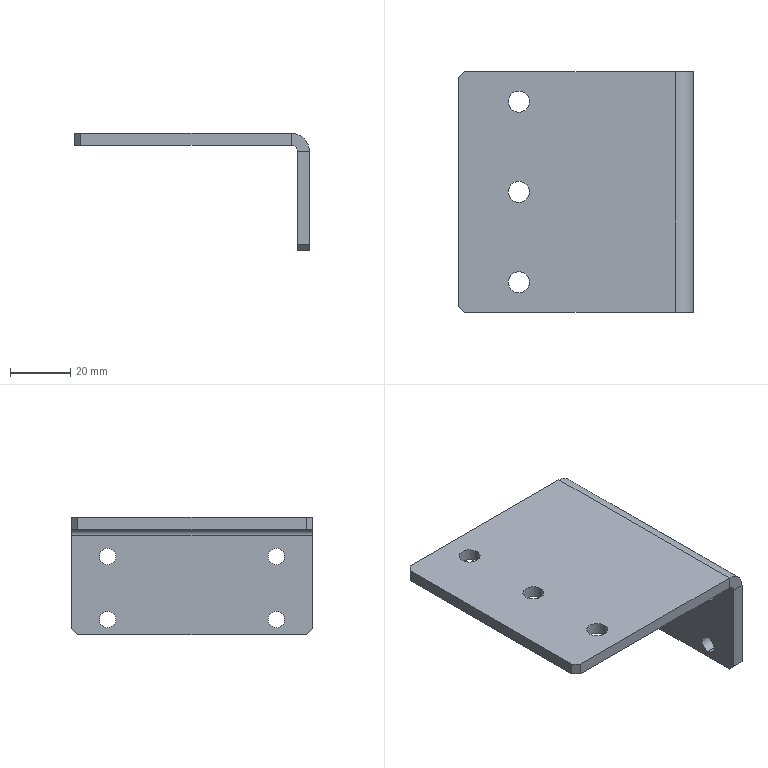Part | NX | features BREP 1 | 1 solid | 32 faces | box 78 x 80 x 39 mm | volume 34737 mm3 | plane 16 | cylinder 16 | commonest cylinder face diameters 5.5 x8 7 x6 4 x1 12 x1
STEP:
#1=CARTESIAN_POINT('',(74.,-38.,-35.));
#2=VERTEX_POINT('',#1);
#3=CARTESIAN_POINT('',(74.,-40.,-33.));
#4=VERTEX_POINT('',#3);
#5=CARTESIAN_POINT('',(74.,-16.5,-56.5));
#6=DIRECTION('',(0.,-0.7071,0.7071));
#7=VECTOR('',#6,1000.);
#8=LINE('',#5,#7);
#9=EDGE_CURVE('',#2,#4,#8,.T.);
#10=ORIENTED_EDGE('',*,*,#9,.F.);
#11=CARTESIAN_POINT('',(78.,-38.,-35.));
#12=VERTEX_POINT('',#11);
#13=CARTESIAN_POINT('',(74.,-38.,-35.));
#14=DIRECTION('',(-1.,0.,0.));
#15=VECTOR('',#14,1000.);
#16=LINE('',#13,#15);
#17=EDGE_CURVE('',#12,#2,#16,.T.);
#18=ORIENTED_EDGE('',*,*,#17,.F.);
#19=CARTESIAN_POINT('',(78.,-40.,-33.));
#20=VERTEX_POINT('',#19);
#21=CARTESIAN_POINT('',(78.,-40.,-33.));
#22=DIRECTION('',(0.,0.7071,-0.7071));
#23=VECTOR('',#22,1000.);
#24=LINE('',#21,#23);
#25=EDGE_CURVE('',#20,#12,#24,.T.);
#26=ORIENTED_EDGE('',*,*,#25,.F.);
#27=CARTESIAN_POINT('',(72.,-40.,-33.));
#28=DIRECTION('',(1.,0.,0.));
#29=VECTOR('',#28,1000.);
#30=LINE('',#27,#29);
#31=EDGE_CURVE('',#4,#20,#30,.T.);
#32=ORIENTED_EDGE('',*,*,#31,.F.);
#33=EDGE_LOOP('',(#10,#18,#26,#32));
#34=FACE_BOUND('',#33,.T.);
#35=CARTESIAN_POINT('',(72.,-40.,-33.));
#36=DIRECTION('',(0.,0.7071,0.7071));
#37=DIRECTION('',(1.,0.,0.));
#38=AXIS2_PLACEMENT_3D('',#35,#36,#37);
#39=PLANE('',#38);
#40=ADVANCED_FACE('',(#34),#39,.F.);
#41=CARTESIAN_POINT('',(74.,40.,-33.));
#42=VERTEX_POINT('',#41);
#43=CARTESIAN_POINT('',(74.,38.,-35.));
#44=VERTEX_POINT('',#43);
#45=CARTESIAN_POINT('',(74.,56.5,-16.5));
#46=DIRECTION('',(0.,-0.7071,-0.7071));
#47=VECTOR('',#46,1000.);
#48=LINE('',#45,#47);
#49=EDGE_CURVE('',#42,#44,#48,.T.);
#50=ORIENTED_EDGE('',*,*,#49,.F.);
#51=CARTESIAN_POINT('',(78.,40.,-33.));
#52=VERTEX_POINT('',#51);
#53=CARTESIAN_POINT('',(72.,40.,-33.));
#54=DIRECTION('',(-1.,0.,0.));
#55=VECTOR('',#54,1000.);
#56=LINE('',#53,#55);
#57=EDGE_CURVE('',#52,#42,#56,.T.);
#58=ORIENTED_EDGE('',*,*,#57,.F.);
#59=CARTESIAN_POINT('',(78.,38.,-35.));
#60=VERTEX_POINT('',#59);
#61=CARTESIAN_POINT('',(78.,38.,-35.));
#62=DIRECTION('',(0.,0.7071,0.7071));
#63=VECTOR('',#62,1000.);
#64=LINE('',#61,#63);
#65=EDGE_CURVE('',#60,#52,#64,.T.);
#66=ORIENTED_EDGE('',*,*,#65,.F.);
#67=CARTESIAN_POINT('',(74.,38.,-35.));
#68=DIRECTION('',(1.,0.,0.));
#69=VECTOR('',#68,1000.);
#70=LINE('',#67,#69);
#71=EDGE_CURVE('',#44,#60,#70,.T.);
#72=ORIENTED_EDGE('',*,*,#71,.F.);
#73=EDGE_LOOP('',(#50,#58,#66,#72));
#74=FACE_BOUND('',#73,.T.);
#75=CARTESIAN_POINT('',(74.,38.,-35.));
#76=DIRECTION('',(0.,-0.7071,0.7071));
#77=DIRECTION('',(1.,0.,0.));
#78=AXIS2_PLACEMENT_3D('',#75,#76,#77);
#79=PLANE('',#78);
#80=ADVANCED_FACE('',(#74),#79,.F.);
#81=CARTESIAN_POINT('',(0.,-38.,4.));
#82=VERTEX_POINT('',#81);
#83=CARTESIAN_POINT('',(2.,-40.,4.));
#84=VERTEX_POINT('',#83);
#85=CARTESIAN_POINT('',(2.,-40.,4.));
#86=DIRECTION('',(0.7071,-0.7071,0.));
#87=VECTOR('',#86,1000.);
#88=LINE('',#85,#87);
#89=EDGE_CURVE('',#82,#84,#88,.T.);
#90=ORIENTED_EDGE('',*,*,#89,.F.);
#91=CARTESIAN_POINT('',(0.,-38.,0.));
#92=VERTEX_POINT('',#91);
#93=CARTESIAN_POINT('',(0.,-38.,4.));
#94=DIRECTION('',(0.,0.,1.));
#95=VECTOR('',#94,1000.);
#96=LINE('',#93,#95);
#97=EDGE_CURVE('',#92,#82,#96,.T.);
#98=ORIENTED_EDGE('',*,*,#97,.F.);
#99=CARTESIAN_POINT('',(2.,-40.,0.));
#100=VERTEX_POINT('',#99);
#101=CARTESIAN_POINT('',(-39.,1.,0.));
#102=DIRECTION('',(-0.7071,0.7071,0.));
#103=VECTOR('',#102,1000.);
#104=LINE('',#101,#103);
#105=EDGE_CURVE('',#100,#92,#104,.T.);
#106=ORIENTED_EDGE('',*,*,#105,.F.);
#107=CARTESIAN_POINT('',(2.,-40.,-2.));
#108=DIRECTION('',(0.,0.,-1.));
#109=VECTOR('',#108,1000.);
#110=LINE('',#107,#109);
#111=EDGE_CURVE('',#84,#100,#110,.T.);
#112=ORIENTED_EDGE('',*,*,#111,.F.);
#113=EDGE_LOOP('',(#90,#98,#106,#112));
#114=FACE_BOUND('',#113,.T.);
#115=CARTESIAN_POINT('',(2.,-40.,-2.));
#116=DIRECTION('',(0.7071,0.7071,0.));
#117=DIRECTION('',(0.,0.,-1.));
#118=AXIS2_PLACEMENT_3D('',#115,#116,#117);
#119=PLANE('',#118);
#120=ADVANCED_FACE('',(#114),#119,.F.);
#121=CARTESIAN_POINT('',(2.,40.,4.));
#122=VERTEX_POINT('',#121);
#123=CARTESIAN_POINT('',(0.,38.,4.));
#124=VERTEX_POINT('',#123);
#125=CARTESIAN_POINT('',(0.,38.,4.));
#126=DIRECTION('',(-0.7071,-0.7071,0.));
#127=VECTOR('',#126,1000.);
#128=LINE('',#125,#127);
#129=EDGE_CURVE('',#122,#124,#128,.T.);
#130=ORIENTED_EDGE('',*,*,#129,.F.);
#131=CARTESIAN_POINT('',(2.,40.,0.));
#132=VERTEX_POINT('',#131);
#133=CARTESIAN_POINT('',(2.,40.,4.));
#134=DIRECTION('',(0.,0.,1.));
#135=VECTOR('',#134,1000.);
#136=LINE('',#133,#135);
#137=EDGE_CURVE('',#132,#122,#136,.T.);
#138=ORIENTED_EDGE('',*,*,#137,.F.);
#139=CARTESIAN_POINT('',(0.,38.,0.));
#140=VERTEX_POINT('',#139);
#141=CARTESIAN_POINT('',(1.,39.,0.));
#142=DIRECTION('',(0.7071,0.7071,0.));
#143=VECTOR('',#142,1000.);
#144=LINE('',#141,#143);
#145=EDGE_CURVE('',#140,#132,#144,.T.);
#146=ORIENTED_EDGE('',*,*,#145,.F.);
#147=CARTESIAN_POINT('',(0.,38.,0.));
#148=DIRECTION('',(0.,0.,-1.));
#149=VECTOR('',#148,1000.);
#150=LINE('',#147,#149);
#151=EDGE_CURVE('',#124,#140,#150,.T.);
#152=ORIENTED_EDGE('',*,*,#151,.F.);
#153=EDGE_LOOP('',(#130,#138,#146,#152));
#154=FACE_BOUND('',#153,.T.);
#155=CARTESIAN_POINT('',(0.,38.,4.));
#156=DIRECTION('',(-0.7071,0.7071,0.));
#157=DIRECTION('',(0.,0.,1.));
#158=AXIS2_PLACEMENT_3D('',#155,#156,#157);
#159=PLANE('',#158);
#160=ADVANCED_FACE('',(#154),#159,.T.);
#161=CARTESIAN_POINT('',(74.,28.,-6.25));
#162=VERTEX_POINT('',#161);
#163=CARTESIAN_POINT('',(78.,28.,-6.25));
#164=VERTEX_POINT('',#163);
#165=CARTESIAN_POINT('',(78.,28.,-6.25));
#166=DIRECTION('',(1.,0.,0.));
#167=VECTOR('',#166,1000.);
#168=LINE('',#165,#167);
#169=EDGE_CURVE('',#162,#164,#168,.T.);
#170=ORIENTED_EDGE('',*,*,#169,.F.);
#171=CARTESIAN_POINT('',(74.,28.,-11.75));
#172=VERTEX_POINT('',#171);
#173=CARTESIAN_POINT('',(74.,28.,-9.));
#174=DIRECTION('',(-1.,0.,0.));
#175=DIRECTION('',(0.,0.,1.));
#176=AXIS2_PLACEMENT_3D('',#173,#174,#175);
#177=CIRCLE('',#176,2.75);
#178=EDGE_CURVE('',#162,#172,#177,.T.);
#179=ORIENTED_EDGE('',*,*,#178,.T.);
#180=CARTESIAN_POINT('',(78.,28.,-11.75));
#181=VERTEX_POINT('',#180);
#182=CARTESIAN_POINT('',(78.,28.,-11.75));
#183=DIRECTION('',(1.,0.,0.));
#184=VECTOR('',#183,1000.);
#185=LINE('',#182,#184);
#186=EDGE_CURVE('',#172,#181,#185,.T.);
#187=ORIENTED_EDGE('',*,*,#186,.T.);
#188=CARTESIAN_POINT('',(78.,28.,-9.));
#189=DIRECTION('',(1.,0.,0.));
#190=DIRECTION('',(0.,0.,-1.));
#191=AXIS2_PLACEMENT_3D('',#188,#189,#190);
#192=CIRCLE('',#191,2.75);
#193=EDGE_CURVE('',#181,#164,#192,.T.);
#194=ORIENTED_EDGE('',*,*,#193,.T.);
#195=EDGE_LOOP('',(#170,#179,#187,#194));
#196=FACE_BOUND('',#195,.T.);
#197=CARTESIAN_POINT('',(78.,28.,-9.));
#198=DIRECTION('',(1.,0.,0.));
#199=DIRECTION('',(0.,0.,-1.));
#200=AXIS2_PLACEMENT_3D('',#197,#198,#199);
#201=CYLINDRICAL_SURFACE('',#200,2.75);
#202=ADVANCED_FACE('',(#196),#201,.F.);
#203=CARTESIAN_POINT('',(74.,28.,-27.25));
#204=VERTEX_POINT('',#203);
#205=CARTESIAN_POINT('',(78.,28.,-27.25));
#206=VERTEX_POINT('',#205);
#207=CARTESIAN_POINT('',(78.,28.,-27.25));
#208=DIRECTION('',(1.,0.,0.));
#209=VECTOR('',#208,1000.);
#210=LINE('',#207,#209);
#211=EDGE_CURVE('',#204,#206,#210,.T.);
#212=ORIENTED_EDGE('',*,*,#211,.F.);
#213=CARTESIAN_POINT('',(74.,28.,-32.75));
#214=VERTEX_POINT('',#213);
#215=CARTESIAN_POINT('',(74.,28.,-30.));
#216=DIRECTION('',(-1.,0.,0.));
#217=DIRECTION('',(0.,0.,1.));
#218=AXIS2_PLACEMENT_3D('',#215,#216,#217);
#219=CIRCLE('',#218,2.75);
#220=EDGE_CURVE('',#204,#214,#219,.T.);
#221=ORIENTED_EDGE('',*,*,#220,.T.);
#222=CARTESIAN_POINT('',(78.,28.,-32.75));
#223=VERTEX_POINT('',#222);
#224=CARTESIAN_POINT('',(78.,28.,-32.75));
#225=DIRECTION('',(1.,0.,0.));
#226=VECTOR('',#225,1000.);
#227=LINE('',#224,#226);
#228=EDGE_CURVE('',#214,#223,#227,.T.);
#229=ORIENTED_EDGE('',*,*,#228,.T.);
#230=CARTESIAN_POINT('',(78.,28.,-30.));
#231=DIRECTION('',(1.,0.,0.));
#232=DIRECTION('',(0.,0.,-1.));
#233=AXIS2_PLACEMENT_3D('',#230,#231,#232);
#234=CIRCLE('',#233,2.75);
#235=EDGE_CURVE('',#223,#206,#234,.T.);
#236=ORIENTED_EDGE('',*,*,#235,.T.);
#237=EDGE_LOOP('',(#212,#221,#229,#236));
#238=FACE_BOUND('',#237,.T.);
#239=CARTESIAN_POINT('',(78.,28.,-30.));
#240=DIRECTION('',(1.,0.,0.));
#241=DIRECTION('',(0.,0.,-1.));
#242=AXIS2_PLACEMENT_3D('',#239,#240,#241);
#243=CYLINDRICAL_SURFACE('',#242,2.75);
#244=ADVANCED_FACE('',(#238),#243,.F.);
#245=CARTESIAN_POINT('',(74.,-28.,-6.25));
#246=VERTEX_POINT('',#245);
#247=CARTESIAN_POINT('',(78.,-28.,-6.25));
#248=VERTEX_POINT('',#247);
#249=CARTESIAN_POINT('',(78.,-28.,-6.25));
#250=DIRECTION('',(1.,0.,0.));
#251=VECTOR('',#250,1000.);
#252=LINE('',#249,#251);
#253=EDGE_CURVE('',#246,#248,#252,.T.);
#254=ORIENTED_EDGE('',*,*,#253,.F.);
#255=CARTESIAN_POINT('',(74.,-28.,-11.75));
#256=VERTEX_POINT('',#255);
#257=CARTESIAN_POINT('',(74.,-28.,-9.));
#258=DIRECTION('',(-1.,0.,0.));
#259=DIRECTION('',(0.,0.,1.));
#260=AXIS2_PLACEMENT_3D('',#257,#258,#259);
#261=CIRCLE('',#260,2.75);
#262=EDGE_CURVE('',#246,#256,#261,.T.);
#263=ORIENTED_EDGE('',*,*,#262,.T.);
#264=CARTESIAN_POINT('',(78.,-28.,-11.75));
#265=VERTEX_POINT('',#264);
#266=CARTESIAN_POINT('',(78.,-28.,-11.75));
#267=DIRECTION('',(1.,0.,0.));
#268=VECTOR('',#267,1000.);
#269=LINE('',#266,#268);
#270=EDGE_CURVE('',#256,#265,#269,.T.);
#271=ORIENTED_EDGE('',*,*,#270,.T.);
#272=CARTESIAN_POINT('',(78.,-28.,-9.));
#273=DIRECTION('',(1.,0.,0.));
#274=DIRECTION('',(0.,0.,-1.));
#275=AXIS2_PLACEMENT_3D('',#272,#273,#274);
#276=CIRCLE('',#275,2.75);
#277=EDGE_CURVE('',#265,#248,#276,.T.);
#278=ORIENTED_EDGE('',*,*,#277,.T.);
#279=EDGE_LOOP('',(#254,#263,#271,#278));
#280=FACE_BOUND('',#279,.T.);
#281=CARTESIAN_POINT('',(78.,-28.,-9.));
#282=DIRECTION('',(1.,0.,0.));
#283=DIRECTION('',(0.,0.,-1.));
#284=AXIS2_PLACEMENT_3D('',#281,#282,#283);
#285=CYLINDRICAL_SURFACE('',#284,2.75);
#286=ADVANCED_FACE('',(#280),#285,.F.);
#287=CARTESIAN_POINT('',(74.,-28.,-27.25));
#288=VERTEX_POINT('',#287);
#289=CARTESIAN_POINT('',(78.,-28.,-27.25));
#290=VERTEX_POINT('',#289);
#291=CARTESIAN_POINT('',(78.,-28.,-27.25));
#292=DIRECTION('',(1.,0.,0.));
#293=VECTOR('',#292,1000.);
#294=LINE('',#291,#293);
#295=EDGE_CURVE('',#288,#290,#294,.T.);
#296=ORIENTED_EDGE('',*,*,#295,.F.);
#297=CARTESIAN_POINT('',(74.,-28.,-32.75));
#298=VERTEX_POINT('',#297);
#299=CARTESIAN_POINT('',(74.,-28.,-30.));
#300=DIRECTION('',(-1.,0.,0.));
#301=DIRECTION('',(0.,0.,1.));
#302=AXIS2_PLACEMENT_3D('',#299,#300,#301);
#303=CIRCLE('',#302,2.75);
#304=EDGE_CURVE('',#288,#298,#303,.T.);
#305=ORIENTED_EDGE('',*,*,#304,.T.);
#306=CARTESIAN_POINT('',(78.,-28.,-32.75));
#307=VERTEX_POINT('',#306);
#308=CARTESIAN_POINT('',(78.,-28.,-32.75));
#309=DIRECTION('',(1.,0.,0.));
#310=VECTOR('',#309,1000.);
#311=LINE('',#308,#310);
#312=EDGE_CURVE('',#298,#307,#311,.T.);
#313=ORIENTED_EDGE('',*,*,#312,.T.);
#314=CARTESIAN_POINT('',(78.,-28.,-30.));
#315=DIRECTION('',(1.,0.,0.));
#316=DIRECTION('',(0.,0.,-1.));
#317=AXIS2_PLACEMENT_3D('',#314,#315,#316);
#318=CIRCLE('',#317,2.75);
#319=EDGE_CURVE('',#307,#290,#318,.T.);
#320=ORIENTED_EDGE('',*,*,#319,.T.);
#321=EDGE_LOOP('',(#296,#305,#313,#320));
#322=FACE_BOUND('',#321,.T.);
#323=CARTESIAN_POINT('',(78.,-28.,-30.));
#324=DIRECTION('',(1.,0.,0.));
#325=DIRECTION('',(0.,0.,-1.));
#326=AXIS2_PLACEMENT_3D('',#323,#324,#325);
#327=CYLINDRICAL_SURFACE('',#326,2.75);
#328=ADVANCED_FACE('',(#322),#327,.F.);
#329=CARTESIAN_POINT('',(16.5,30.,4.));
#330=VERTEX_POINT('',#329);
#331=CARTESIAN_POINT('',(16.5,30.,0.));
#332=VERTEX_POINT('',#331);
#333=CARTESIAN_POINT('',(16.5,30.,4.));
#334=DIRECTION('',(0.,0.,1.));
#335=VECTOR('',#334,1000.);
#336=LINE('',#333,#335);
#337=EDGE_CURVE('',#330,#332,#336,.F.);
#338=ORIENTED_EDGE('',*,*,#337,.T.);
#339=CARTESIAN_POINT('',(23.5,30.,0.));
#340=VERTEX_POINT('',#339);
#341=CARTESIAN_POINT('',(20.,30.,0.));
#342=DIRECTION('',(0.,0.,-1.));
#343=DIRECTION('',(-1.,0.,0.));
#344=AXIS2_PLACEMENT_3D('',#341,#342,#343);
#345=CIRCLE('',#344,3.5);
#346=EDGE_CURVE('',#332,#340,#345,.T.);
#347=ORIENTED_EDGE('',*,*,#346,.T.);
#348=CARTESIAN_POINT('',(23.5,30.,4.));
#349=VERTEX_POINT('',#348);
#350=CARTESIAN_POINT('',(23.5,30.,4.));
#351=DIRECTION('',(0.,0.,1.));
#352=VECTOR('',#351,1000.);
#353=LINE('',#350,#352);
#354=EDGE_CURVE('',#349,#340,#353,.F.);
#355=ORIENTED_EDGE('',*,*,#354,.F.);
#356=CARTESIAN_POINT('',(20.,30.,4.));
#357=DIRECTION('',(0.,0.,1.));
#358=DIRECTION('',(1.,0.,0.));
#359=AXIS2_PLACEMENT_3D('',#356,#357,#358);
#360=CIRCLE('',#359,3.5);
#361=EDGE_CURVE('',#349,#330,#360,.T.);
#362=ORIENTED_EDGE('',*,*,#361,.T.);
#363=EDGE_LOOP('',(#338,#347,#355,#362));
#364=FACE_BOUND('',#363,.T.);
#365=CARTESIAN_POINT('',(20.,30.,4.));
#366=DIRECTION('',(0.,0.,1.));
#367=DIRECTION('',(1.,0.,0.));
#368=AXIS2_PLACEMENT_3D('',#365,#366,#367);
#369=CYLINDRICAL_SURFACE('',#368,3.5);
#370=ADVANCED_FACE('',(#364),#369,.F.);
#371=CARTESIAN_POINT('',(16.5,0.,4.));
#372=VERTEX_POINT('',#371);
#373=CARTESIAN_POINT('',(16.5,0.,0.));
#374=VERTEX_POINT('',#373);
#375=CARTESIAN_POINT('',(16.5,0.,4.));
#376=DIRECTION('',(0.,0.,1.));
#377=VECTOR('',#376,1000.);
#378=LINE('',#375,#377);
#379=EDGE_CURVE('',#372,#374,#378,.F.);
#380=ORIENTED_EDGE('',*,*,#379,.T.);
#381=CARTESIAN_POINT('',(23.5,0.,0.));
#382=VERTEX_POINT('',#381);
#383=CARTESIAN_POINT('',(20.,0.,0.));
#384=DIRECTION('',(0.,0.,-1.));
#385=DIRECTION('',(-1.,0.,0.));
#386=AXIS2_PLACEMENT_3D('',#383,#384,#385);
#387=CIRCLE('',#386,3.5);
#388=EDGE_CURVE('',#374,#382,#387,.T.);
#389=ORIENTED_EDGE('',*,*,#388,.T.);
#390=CARTESIAN_POINT('',(23.5,0.,4.));
#391=VERTEX_POINT('',#390);
#392=CARTESIAN_POINT('',(23.5,0.,4.));
#393=DIRECTION('',(0.,0.,1.));
#394=VECTOR('',#393,1000.);
#395=LINE('',#392,#394);
#396=EDGE_CURVE('',#391,#382,#395,.F.);
#397=ORIENTED_EDGE('',*,*,#396,.F.);
#398=CARTESIAN_POINT('',(20.,0.,4.));
#399=DIRECTION('',(0.,0.,1.));
#400=DIRECTION('',(1.,0.,0.));
#401=AXIS2_PLACEMENT_3D('',#398,#399,#400);
#402=CIRCLE('',#401,3.5);
#403=EDGE_CURVE('',#391,#372,#402,.T.);
#404=ORIENTED_EDGE('',*,*,#403,.T.);
#405=EDGE_LOOP('',(#380,#389,#397,#404));
#406=FACE_BOUND('',#405,.T.);
#407=CARTESIAN_POINT('',(20.,0.,4.));
#408=DIRECTION('',(0.,0.,1.));
#409=DIRECTION('',(1.,0.,0.));
#410=AXIS2_PLACEMENT_3D('',#407,#408,#409);
#411=CYLINDRICAL_SURFACE('',#410,3.5);
#412=ADVANCED_FACE('',(#406),#411,.F.);
#413=CARTESIAN_POINT('',(16.5,-30.,4.));
#414=VERTEX_POINT('',#413);
#415=CARTESIAN_POINT('',(16.5,-30.,0.));
#416=VERTEX_POINT('',#415);
#417=CARTESIAN_POINT('',(16.5,-30.,4.));
#418=DIRECTION('',(0.,0.,1.));
#419=VECTOR('',#418,1000.);
#420=LINE('',#417,#419);
#421=EDGE_CURVE('',#414,#416,#420,.F.);
#422=ORIENTED_EDGE('',*,*,#421,.T.);
#423=CARTESIAN_POINT('',(23.5,-30.,0.));
#424=VERTEX_POINT('',#423);
#425=CARTESIAN_POINT('',(20.,-30.,0.));
#426=DIRECTION('',(0.,0.,-1.));
#427=DIRECTION('',(-1.,0.,0.));
#428=AXIS2_PLACEMENT_3D('',#425,#426,#427);
#429=CIRCLE('',#428,3.5);
#430=EDGE_CURVE('',#416,#424,#429,.T.);
#431=ORIENTED_EDGE('',*,*,#430,.T.);
#432=CARTESIAN_POINT('',(23.5,-30.,4.));
#433=VERTEX_POINT('',#432);
#434=CARTESIAN_POINT('',(23.5,-30.,4.));
#435=DIRECTION('',(0.,0.,1.));
#436=VECTOR('',#435,1000.);
#437=LINE('',#434,#436);
#438=EDGE_CURVE('',#433,#424,#437,.F.);
#439=ORIENTED_EDGE('',*,*,#438,.F.);
#440=CARTESIAN_POINT('',(20.,-30.,4.));
#441=DIRECTION('',(0.,0.,1.));
#442=DIRECTION('',(1.,0.,0.));
#443=AXIS2_PLACEMENT_3D('',#440,#441,#442);
#444=CIRCLE('',#443,3.5);
#445=EDGE_CURVE('',#433,#414,#444,.T.);
#446=ORIENTED_EDGE('',*,*,#445,.T.);
#447=EDGE_LOOP('',(#422,#431,#439,#446));
#448=FACE_BOUND('',#447,.T.);
#449=CARTESIAN_POINT('',(20.,-30.,4.));
#450=DIRECTION('',(0.,0.,1.));
#451=DIRECTION('',(1.,0.,0.));
#452=AXIS2_PLACEMENT_3D('',#449,#450,#451);
#453=CYLINDRICAL_SURFACE('',#452,3.5);
#454=ADVANCED_FACE('',(#448),#453,.F.);
#455=CARTESIAN_POINT('',(74.,-40.,-2.));
#456=VERTEX_POINT('',#455);
#457=CARTESIAN_POINT('',(74.,-40.,0.));
#458=DIRECTION('',(0.,0.,-1.));
#459=VECTOR('',#458,1000.);
#460=LINE('',#457,#459);
#461=EDGE_CURVE('',#456,#4,#460,.T.);
#462=ORIENTED_EDGE('',*,*,#461,.T.);
#463=ORIENTED_EDGE('',*,*,#31,.T.);
#464=CARTESIAN_POINT('',(78.,-40.,-2.));
#465=VERTEX_POINT('',#464);
#466=CARTESIAN_POINT('',(78.,-40.,0.));
#467=DIRECTION('',(0.,0.,-1.));
#468=VECTOR('',#467,1000.);
#469=LINE('',#466,#468);
#470=EDGE_CURVE('',#465,#20,#469,.T.);
#471=ORIENTED_EDGE('',*,*,#470,.F.);
#472=CARTESIAN_POINT('',(78.,-40.,-2.));
#473=DIRECTION('',(-1.,0.,0.));
#474=VECTOR('',#473,1000.);
#475=LINE('',#472,#474);
#476=EDGE_CURVE('',#465,#456,#475,.T.);
#477=ORIENTED_EDGE('',*,*,#476,.T.);
#478=EDGE_LOOP('',(#462,#463,#471,#477));
#479=FACE_BOUND('',#478,.T.);
#480=CARTESIAN_POINT('',(72.,-40.,-2.));
#481=DIRECTION('',(0.,-1.,0.));
#482=DIRECTION('',(-1.,0.,0.));
#483=AXIS2_PLACEMENT_3D('',#480,#481,#482);
#484=PLANE('',#483);
#485=ADVANCED_FACE('',(#479),#484,.T.);
#486=CARTESIAN_POINT('',(72.,40.,0.));
#487=VERTEX_POINT('',#486);
#488=CARTESIAN_POINT('',(0.,40.,0.));
#489=DIRECTION('',(1.,0.,0.));
#490=VECTOR('',#489,1000.);
#491=LINE('',#488,#490);
#492=EDGE_CURVE('',#132,#487,#491,.T.);
#493=ORIENTED_EDGE('',*,*,#492,.F.);
#494=ORIENTED_EDGE('',*,*,#137,.T.);
#495=CARTESIAN_POINT('',(72.,40.,4.));
#496=VERTEX_POINT('',#495);
#497=CARTESIAN_POINT('',(0.,40.,4.));
#498=DIRECTION('',(1.,0.,0.));
#499=VECTOR('',#498,1000.);
#500=LINE('',#497,#499);
#501=EDGE_CURVE('',#122,#496,#500,.T.);
#502=ORIENTED_EDGE('',*,*,#501,.T.);
#503=CARTESIAN_POINT('',(72.,40.,4.));
#504=DIRECTION('',(0.,0.,-1.));
#505=VECTOR('',#504,1000.);
#506=LINE('',#503,#505);
#507=EDGE_CURVE('',#496,#487,#506,.T.);
#508=ORIENTED_EDGE('',*,*,#507,.T.);
#509=EDGE_LOOP('',(#493,#494,#502,#508));
#510=FACE_BOUND('',#509,.T.);
#511=CARTESIAN_POINT('',(72.,40.,-2.));
#512=DIRECTION('',(0.,-1.,0.));
#513=DIRECTION('',(-1.,0.,0.));
#514=AXIS2_PLACEMENT_3D('',#511,#512,#513);
#515=PLANE('',#514);
#516=ADVANCED_FACE('',(#510),#515,.F.);
#517=CARTESIAN_POINT('',(72.,-40.,4.));
#518=VERTEX_POINT('',#517);
#519=CARTESIAN_POINT('',(72.,-40.,-2.));
#520=DIRECTION('',(0.,1.,0.));
#521=DIRECTION('',(1.,0.,0.));
#522=AXIS2_PLACEMENT_3D('',#519,#520,#521);
#523=CIRCLE('',#522,6.);
#524=EDGE_CURVE('',#518,#465,#523,.T.);
#525=ORIENTED_EDGE('',*,*,#524,.T.);
#526=CARTESIAN_POINT('',(78.,40.,-2.));
#527=VERTEX_POINT('',#526);
#528=CARTESIAN_POINT('',(78.,40.,-2.));
#529=DIRECTION('',(0.,-1.,0.));
#530=VECTOR('',#529,1000.);
#531=LINE('',#528,#530);
#532=EDGE_CURVE('',#527,#465,#531,.T.);
#533=ORIENTED_EDGE('',*,*,#532,.F.);
#534=CARTESIAN_POINT('',(72.,40.,-2.));
#535=DIRECTION('',(0.,1.,0.));
#536=DIRECTION('',(1.,0.,0.));
#537=AXIS2_PLACEMENT_3D('',#534,#535,#536);
#538=CIRCLE('',#537,6.);
#539=EDGE_CURVE('',#496,#527,#538,.T.);
#540=ORIENTED_EDGE('',*,*,#539,.F.);
#541=CARTESIAN_POINT('',(72.,40.,4.));
#542=DIRECTION('',(0.,-1.,0.));
#543=VECTOR('',#542,1000.);
#544=LINE('',#541,#543);
#545=EDGE_CURVE('',#496,#518,#544,.T.);
#546=ORIENTED_EDGE('',*,*,#545,.T.);
#547=EDGE_LOOP('',(#525,#533,#540,#546));
#548=FACE_BOUND('',#547,.T.);
#549=CARTESIAN_POINT('',(72.,40.,-2.));
#550=DIRECTION('',(0.,-1.,0.));
#551=DIRECTION('',(0.,0.,-1.));
#552=AXIS2_PLACEMENT_3D('',#549,#550,#551);
#553=CYLINDRICAL_SURFACE('',#552,6.);
#554=ADVANCED_FACE('',(#548),#553,.T.);
#555=ORIENTED_EDGE('',*,*,#501,.F.);
#556=ORIENTED_EDGE('',*,*,#129,.T.);
#557=CARTESIAN_POINT('',(0.,40.,4.));
#558=DIRECTION('',(0.,-1.,0.));
#559=VECTOR('',#558,1000.);
#560=LINE('',#557,#559);
#561=EDGE_CURVE('',#124,#82,#560,.T.);
#562=ORIENTED_EDGE('',*,*,#561,.T.);
#563=ORIENTED_EDGE('',*,*,#89,.T.);
#564=CARTESIAN_POINT('',(0.,-40.,4.));
#565=DIRECTION('',(1.,0.,0.));
#566=VECTOR('',#565,1000.);
#567=LINE('',#564,#566);
#568=EDGE_CURVE('',#84,#518,#567,.T.);
#569=ORIENTED_EDGE('',*,*,#568,.T.);
#570=ORIENTED_EDGE('',*,*,#545,.F.);
#571=EDGE_LOOP('',(#555,#556,#562,#563,#569,#570));
#572=FACE_BOUND('',#571,.T.);
#573=ORIENTED_EDGE('',*,*,#445,.F.);
#574=CARTESIAN_POINT('',(20.,-30.,4.));
#575=DIRECTION('',(0.,0.,1.));
#576=DIRECTION('',(1.,0.,0.));
#577=AXIS2_PLACEMENT_3D('',#574,#575,#576);
#578=CIRCLE('',#577,3.5);
#579=EDGE_CURVE('',#414,#433,#578,.T.);
#580=ORIENTED_EDGE('',*,*,#579,.F.);
#581=EDGE_LOOP('',(#573,#580));
#582=FACE_BOUND('',#581,.T.);
#583=ORIENTED_EDGE('',*,*,#403,.F.);
#584=CARTESIAN_POINT('',(20.,0.,4.));
#585=DIRECTION('',(0.,0.,1.));
#586=DIRECTION('',(1.,0.,0.));
#587=AXIS2_PLACEMENT_3D('',#584,#585,#586);
#588=CIRCLE('',#587,3.5);
#589=EDGE_CURVE('',#372,#391,#588,.T.);
#590=ORIENTED_EDGE('',*,*,#589,.F.);
#591=EDGE_LOOP('',(#583,#590));
#592=FACE_BOUND('',#591,.T.);
#593=ORIENTED_EDGE('',*,*,#361,.F.);
#594=CARTESIAN_POINT('',(20.,30.,4.));
#595=DIRECTION('',(0.,0.,1.));
#596=DIRECTION('',(1.,0.,0.));
#597=AXIS2_PLACEMENT_3D('',#594,#595,#596);
#598=CIRCLE('',#597,3.5);
#599=EDGE_CURVE('',#330,#349,#598,.T.);
#600=ORIENTED_EDGE('',*,*,#599,.F.);
#601=EDGE_LOOP('',(#593,#600));
#602=FACE_BOUND('',#601,.T.);
#603=CARTESIAN_POINT('',(0.,40.,4.));
#604=DIRECTION('',(0.,0.,-1.));
#605=DIRECTION('',(-1.,0.,0.));
#606=AXIS2_PLACEMENT_3D('',#603,#604,#605);
#607=PLANE('',#606);
#608=ADVANCED_FACE('',(#572,#582,#592,#602),#607,.F.);
#609=ORIENTED_EDGE('',*,*,#561,.F.);
#610=ORIENTED_EDGE('',*,*,#151,.T.);
#611=CARTESIAN_POINT('',(0.,40.,0.));
#612=DIRECTION('',(0.,-1.,0.));
#613=VECTOR('',#612,1000.);
#614=LINE('',#611,#613);
#615=EDGE_CURVE('',#140,#92,#614,.T.);
#616=ORIENTED_EDGE('',*,*,#615,.T.);
#617=ORIENTED_EDGE('',*,*,#97,.T.);
#618=EDGE_LOOP('',(#609,#610,#616,#617));
#619=FACE_BOUND('',#618,.T.);
#620=CARTESIAN_POINT('',(0.,40.,4.));
#621=DIRECTION('',(-1.,0.,0.));
#622=DIRECTION('',(0.,0.,1.));
#623=AXIS2_PLACEMENT_3D('',#620,#621,#622);
#624=PLANE('',#623);
#625=ADVANCED_FACE('',(#619),#624,.T.);
#626=ORIENTED_EDGE('',*,*,#615,.F.);
#627=ORIENTED_EDGE('',*,*,#145,.T.);
#628=ORIENTED_EDGE('',*,*,#492,.T.);
#629=CARTESIAN_POINT('',(72.,-40.,0.));
#630=VERTEX_POINT('',#629);
#631=CARTESIAN_POINT('',(72.,40.,0.));
#632=DIRECTION('',(0.,-1.,0.));
#633=VECTOR('',#632,1000.);
#634=LINE('',#631,#633);
#635=EDGE_CURVE('',#487,#630,#634,.T.);
#636=ORIENTED_EDGE('',*,*,#635,.T.);
#637=CARTESIAN_POINT('',(0.,-40.,0.));
#638=DIRECTION('',(1.,0.,0.));
#639=VECTOR('',#638,1000.);
#640=LINE('',#637,#639);
#641=EDGE_CURVE('',#100,#630,#640,.T.);
#642=ORIENTED_EDGE('',*,*,#641,.F.);
#643=ORIENTED_EDGE('',*,*,#105,.T.);
#644=EDGE_LOOP('',(#626,#627,#628,#636,#642,#643));
#645=FACE_BOUND('',#644,.T.);
#646=CARTESIAN_POINT('',(20.,-30.,0.));
#647=DIRECTION('',(0.,0.,-1.));
#648=DIRECTION('',(-1.,0.,0.));
#649=AXIS2_PLACEMENT_3D('',#646,#647,#648);
#650=CIRCLE('',#649,3.5);
#651=EDGE_CURVE('',#424,#416,#650,.T.);
#652=ORIENTED_EDGE('',*,*,#651,.F.);
#653=ORIENTED_EDGE('',*,*,#430,.F.);
#654=EDGE_LOOP('',(#652,#653));
#655=FACE_BOUND('',#654,.T.);
#656=CARTESIAN_POINT('',(20.,0.,0.));
#657=DIRECTION('',(0.,0.,-1.));
#658=DIRECTION('',(-1.,0.,0.));
#659=AXIS2_PLACEMENT_3D('',#656,#657,#658);
#660=CIRCLE('',#659,3.5);
#661=EDGE_CURVE('',#382,#374,#660,.T.);
#662=ORIENTED_EDGE('',*,*,#661,.F.);
#663=ORIENTED_EDGE('',*,*,#388,.F.);
#664=EDGE_LOOP('',(#662,#663));
#665=FACE_BOUND('',#664,.T.);
#666=CARTESIAN_POINT('',(20.,30.,0.));
#667=DIRECTION('',(0.,0.,-1.));
#668=DIRECTION('',(-1.,0.,0.));
#669=AXIS2_PLACEMENT_3D('',#666,#667,#668);
#670=CIRCLE('',#669,3.5);
#671=EDGE_CURVE('',#340,#332,#670,.T.);
#672=ORIENTED_EDGE('',*,*,#671,.F.);
#673=ORIENTED_EDGE('',*,*,#346,.F.);
#674=EDGE_LOOP('',(#672,#673));
#675=FACE_BOUND('',#674,.T.);
#676=CARTESIAN_POINT('',(0.,40.,0.));
#677=DIRECTION('',(0.,0.,-1.));
#678=DIRECTION('',(-1.,0.,0.));
#679=AXIS2_PLACEMENT_3D('',#676,#677,#678);
#680=PLANE('',#679);
#681=ADVANCED_FACE('',(#645,#655,#665,#675),#680,.T.);
#682=CARTESIAN_POINT('',(72.,-40.,-2.));
#683=DIRECTION('',(0.,1.,0.));
#684=DIRECTION('',(0.,0.,-1.));
#685=AXIS2_PLACEMENT_3D('',#682,#683,#684);
#686=CIRCLE('',#685,2.);
#687=EDGE_CURVE('',#630,#456,#686,.T.);
#688=ORIENTED_EDGE('',*,*,#687,.F.);
#689=ORIENTED_EDGE('',*,*,#635,.F.);
#690=CARTESIAN_POINT('',(74.,40.,-2.));
#691=VERTEX_POINT('',#690);
#692=CARTESIAN_POINT('',(72.,40.,-2.));
#693=DIRECTION('',(0.,1.,0.));
#694=DIRECTION('',(0.,0.,-1.));
#695=AXIS2_PLACEMENT_3D('',#692,#693,#694);
#696=CIRCLE('',#695,2.);
#697=EDGE_CURVE('',#487,#691,#696,.T.);
#698=ORIENTED_EDGE('',*,*,#697,.T.);
#699=CARTESIAN_POINT('',(74.,40.,-2.));
#700=DIRECTION('',(0.,-1.,0.));
#701=VECTOR('',#700,1000.);
#702=LINE('',#699,#701);
#703=EDGE_CURVE('',#691,#456,#702,.T.);
#704=ORIENTED_EDGE('',*,*,#703,.T.);
#705=EDGE_LOOP('',(#688,#689,#698,#704));
#706=FACE_BOUND('',#705,.T.);
#707=CARTESIAN_POINT('',(72.,40.,-2.));
#708=DIRECTION('',(0.,-1.,0.));
#709=DIRECTION('',(0.,0.,-1.));
#710=AXIS2_PLACEMENT_3D('',#707,#708,#709);
#711=CYLINDRICAL_SURFACE('',#710,2.);
#712=ADVANCED_FACE('',(#706),#711,.F.);
#713=CARTESIAN_POINT('',(74.,40.,0.));
#714=DIRECTION('',(0.,0.,-1.));
#715=VECTOR('',#714,1000.);
#716=LINE('',#713,#715);
#717=EDGE_CURVE('',#691,#42,#716,.T.);
#718=ORIENTED_EDGE('',*,*,#717,.T.);
#719=ORIENTED_EDGE('',*,*,#49,.T.);
#720=CARTESIAN_POINT('',(74.,40.,-35.));
#721=DIRECTION('',(0.,-1.,0.));
#722=VECTOR('',#721,1000.);
#723=LINE('',#720,#722);
#724=EDGE_CURVE('',#44,#2,#723,.T.);
#725=ORIENTED_EDGE('',*,*,#724,.T.);
#726=ORIENTED_EDGE('',*,*,#9,.T.);
#727=ORIENTED_EDGE('',*,*,#461,.F.);
#728=ORIENTED_EDGE('',*,*,#703,.F.);
#729=EDGE_LOOP('',(#718,#719,#725,#726,#727,#728));
#730=FACE_BOUND('',#729,.T.);
#731=CARTESIAN_POINT('',(74.,-28.,-30.));
#732=DIRECTION('',(-1.,0.,0.));
#733=DIRECTION('',(0.,0.,1.));
#734=AXIS2_PLACEMENT_3D('',#731,#732,#733);
#735=CIRCLE('',#734,2.75);
#736=EDGE_CURVE('',#298,#288,#735,.T.);
#737=ORIENTED_EDGE('',*,*,#736,.F.);
#738=ORIENTED_EDGE('',*,*,#304,.F.);
#739=EDGE_LOOP('',(#737,#738));
#740=FACE_BOUND('',#739,.T.);
#741=CARTESIAN_POINT('',(74.,-28.,-9.));
#742=DIRECTION('',(-1.,0.,0.));
#743=DIRECTION('',(0.,0.,1.));
#744=AXIS2_PLACEMENT_3D('',#741,#742,#743);
#745=CIRCLE('',#744,2.75);
#746=EDGE_CURVE('',#256,#246,#745,.T.);
#747=ORIENTED_EDGE('',*,*,#746,.F.);
#748=ORIENTED_EDGE('',*,*,#262,.F.);
#749=EDGE_LOOP('',(#747,#748));
#750=FACE_BOUND('',#749,.T.);
#751=CARTESIAN_POINT('',(74.,28.,-30.));
#752=DIRECTION('',(-1.,0.,0.));
#753=DIRECTION('',(0.,0.,1.));
#754=AXIS2_PLACEMENT_3D('',#751,#752,#753);
#755=CIRCLE('',#754,2.75);
#756=EDGE_CURVE('',#214,#204,#755,.T.);
#757=ORIENTED_EDGE('',*,*,#756,.F.);
#758=ORIENTED_EDGE('',*,*,#220,.F.);
#759=EDGE_LOOP('',(#757,#758));
#760=FACE_BOUND('',#759,.T.);
#761=CARTESIAN_POINT('',(74.,28.,-9.));
#762=DIRECTION('',(-1.,0.,0.));
#763=DIRECTION('',(0.,0.,1.));
#764=AXIS2_PLACEMENT_3D('',#761,#762,#763);
#765=CIRCLE('',#764,2.75);
#766=EDGE_CURVE('',#172,#162,#765,.T.);
#767=ORIENTED_EDGE('',*,*,#766,.F.);
#768=ORIENTED_EDGE('',*,*,#178,.F.);
#769=EDGE_LOOP('',(#767,#768));
#770=FACE_BOUND('',#769,.T.);
#771=CARTESIAN_POINT('',(74.,40.,0.));
#772=DIRECTION('',(-1.,0.,0.));
#773=DIRECTION('',(0.,0.,1.));
#774=AXIS2_PLACEMENT_3D('',#771,#772,#773);
#775=PLANE('',#774);
#776=ADVANCED_FACE('',(#730,#740,#750,#760,#770),#775,.T.);
#777=ORIENTED_EDGE('',*,*,#724,.F.);
#778=ORIENTED_EDGE('',*,*,#71,.T.);
#779=CARTESIAN_POINT('',(78.,40.,-35.));
#780=DIRECTION('',(0.,-1.,0.));
#781=VECTOR('',#780,1000.);
#782=LINE('',#779,#781);
#783=EDGE_CURVE('',#60,#12,#782,.T.);
#784=ORIENTED_EDGE('',*,*,#783,.T.);
#785=ORIENTED_EDGE('',*,*,#17,.T.);
#786=EDGE_LOOP('',(#777,#778,#784,#785));
#787=FACE_BOUND('',#786,.T.);
#788=CARTESIAN_POINT('',(74.,40.,-35.));
#789=DIRECTION('',(0.,0.,-1.));
#790=DIRECTION('',(-1.,0.,0.));
#791=AXIS2_PLACEMENT_3D('',#788,#789,#790);
#792=PLANE('',#791);
#793=ADVANCED_FACE('',(#787),#792,.T.);
#794=ORIENTED_EDGE('',*,*,#783,.F.);
#795=ORIENTED_EDGE('',*,*,#65,.T.);
#796=CARTESIAN_POINT('',(78.,40.,0.));
#797=DIRECTION('',(0.,0.,-1.));
#798=VECTOR('',#797,1000.);
#799=LINE('',#796,#798);
#800=EDGE_CURVE('',#527,#52,#799,.T.);
#801=ORIENTED_EDGE('',*,*,#800,.F.);
#802=ORIENTED_EDGE('',*,*,#532,.T.);
#803=ORIENTED_EDGE('',*,*,#470,.T.);
#804=ORIENTED_EDGE('',*,*,#25,.T.);
#805=EDGE_LOOP('',(#794,#795,#801,#802,#803,#804));
#806=FACE_BOUND('',#805,.T.);
#807=ORIENTED_EDGE('',*,*,#319,.F.);
#808=CARTESIAN_POINT('',(78.,-28.,-30.));
#809=DIRECTION('',(1.,0.,0.));
#810=DIRECTION('',(0.,0.,-1.));
#811=AXIS2_PLACEMENT_3D('',#808,#809,#810);
#812=CIRCLE('',#811,2.75);
#813=EDGE_CURVE('',#290,#307,#812,.T.);
#814=ORIENTED_EDGE('',*,*,#813,.F.);
#815=EDGE_LOOP('',(#807,#814));
#816=FACE_BOUND('',#815,.T.);
#817=ORIENTED_EDGE('',*,*,#277,.F.);
#818=CARTESIAN_POINT('',(78.,-28.,-9.));
#819=DIRECTION('',(1.,0.,0.));
#820=DIRECTION('',(0.,0.,-1.));
#821=AXIS2_PLACEMENT_3D('',#818,#819,#820);
#822=CIRCLE('',#821,2.75);
#823=EDGE_CURVE('',#248,#265,#822,.T.);
#824=ORIENTED_EDGE('',*,*,#823,.F.);
#825=EDGE_LOOP('',(#817,#824));
#826=FACE_BOUND('',#825,.T.);
#827=ORIENTED_EDGE('',*,*,#235,.F.);
#828=CARTESIAN_POINT('',(78.,28.,-30.));
#829=DIRECTION('',(1.,0.,0.));
#830=DIRECTION('',(0.,0.,-1.));
#831=AXIS2_PLACEMENT_3D('',#828,#829,#830);
#832=CIRCLE('',#831,2.75);
#833=EDGE_CURVE('',#206,#223,#832,.T.);
#834=ORIENTED_EDGE('',*,*,#833,.F.);
#835=EDGE_LOOP('',(#827,#834));
#836=FACE_BOUND('',#835,.T.);
#837=ORIENTED_EDGE('',*,*,#193,.F.);
#838=CARTESIAN_POINT('',(78.,28.,-9.));
#839=DIRECTION('',(1.,0.,0.));
#840=DIRECTION('',(0.,0.,-1.));
#841=AXIS2_PLACEMENT_3D('',#838,#839,#840);
#842=CIRCLE('',#841,2.75);
#843=EDGE_CURVE('',#164,#181,#842,.T.);
#844=ORIENTED_EDGE('',*,*,#843,.F.);
#845=EDGE_LOOP('',(#837,#844));
#846=FACE_BOUND('',#845,.T.);
#847=CARTESIAN_POINT('',(78.,40.,0.));
#848=DIRECTION('',(-1.,0.,0.));
#849=DIRECTION('',(0.,0.,1.));
#850=AXIS2_PLACEMENT_3D('',#847,#848,#849);
#851=PLANE('',#850);
#852=ADVANCED_FACE('',(#806,#816,#826,#836,#846),#851,.F.);
#853=ORIENTED_EDGE('',*,*,#568,.F.);
#854=ORIENTED_EDGE('',*,*,#111,.T.);
#855=ORIENTED_EDGE('',*,*,#641,.T.);
#856=CARTESIAN_POINT('',(72.,-40.,0.));
#857=DIRECTION('',(0.,0.,1.));
#858=VECTOR('',#857,1000.);
#859=LINE('',#856,#858);
#860=EDGE_CURVE('',#630,#518,#859,.T.);
#861=ORIENTED_EDGE('',*,*,#860,.T.);
#862=EDGE_LOOP('',(#853,#854,#855,#861));
#863=FACE_BOUND('',#862,.T.);
#864=CARTESIAN_POINT('',(78.,-40.,-2.));
#865=DIRECTION('',(0.,-1.,0.));
#866=DIRECTION('',(0.,0.,-1.));
#867=AXIS2_PLACEMENT_3D('',#864,#865,#866);
#868=PLANE('',#867);
#869=ADVANCED_FACE('',(#863),#868,.T.);
#870=ORIENTED_EDGE('',*,*,#860,.F.);
#871=ORIENTED_EDGE('',*,*,#687,.T.);
#872=ORIENTED_EDGE('',*,*,#476,.F.);
#873=ORIENTED_EDGE('',*,*,#524,.F.);
#874=EDGE_LOOP('',(#870,#871,#872,#873));
#875=FACE_BOUND('',#874,.T.);
#876=CARTESIAN_POINT('',(72.,-40.,0.));
#877=DIRECTION('',(0.,-1.,0.));
#878=DIRECTION('',(0.,0.,-1.));
#879=AXIS2_PLACEMENT_3D('',#876,#877,#878);
#880=PLANE('',#879);
#881=ADVANCED_FACE('',(#875),#880,.T.);
#882=ORIENTED_EDGE('',*,*,#800,.T.);
#883=ORIENTED_EDGE('',*,*,#57,.T.);
#884=ORIENTED_EDGE('',*,*,#717,.F.);
#885=CARTESIAN_POINT('',(74.,40.,-2.));
#886=DIRECTION('',(1.,0.,0.));
#887=VECTOR('',#886,1000.);
#888=LINE('',#885,#887);
#889=EDGE_CURVE('',#691,#527,#888,.T.);
#890=ORIENTED_EDGE('',*,*,#889,.T.);
#891=EDGE_LOOP('',(#882,#883,#884,#890));
#892=FACE_BOUND('',#891,.T.);
#893=CARTESIAN_POINT('',(72.,40.,4.));
#894=DIRECTION('',(0.,1.,0.));
#895=DIRECTION('',(0.,0.,1.));
#896=AXIS2_PLACEMENT_3D('',#893,#894,#895);
#897=PLANE('',#896);
#898=ADVANCED_FACE('',(#892),#897,.T.);
#899=ORIENTED_EDGE('',*,*,#889,.F.);
#900=ORIENTED_EDGE('',*,*,#697,.F.);
#901=ORIENTED_EDGE('',*,*,#507,.F.);
#902=ORIENTED_EDGE('',*,*,#539,.T.);
#903=EDGE_LOOP('',(#899,#900,#901,#902));
#904=FACE_BOUND('',#903,.T.);
#905=CARTESIAN_POINT('',(74.,40.,-2.));
#906=DIRECTION('',(0.,1.,0.));
#907=DIRECTION('',(0.,0.,1.));
#908=AXIS2_PLACEMENT_3D('',#905,#906,#907);
#909=PLANE('',#908);
#910=ADVANCED_FACE('',(#904),#909,.T.);
#911=ORIENTED_EDGE('',*,*,#651,.T.);
#912=ORIENTED_EDGE('',*,*,#421,.F.);
#913=ORIENTED_EDGE('',*,*,#579,.T.);
#914=ORIENTED_EDGE('',*,*,#438,.T.);
#915=EDGE_LOOP('',(#911,#912,#913,#914));
#916=FACE_BOUND('',#915,.T.);
#917=CARTESIAN_POINT('',(20.,-30.,4.));
#918=DIRECTION('',(0.,0.,1.));
#919=DIRECTION('',(1.,0.,0.));
#920=AXIS2_PLACEMENT_3D('',#917,#918,#919);
#921=CYLINDRICAL_SURFACE('',#920,3.5);
#922=ADVANCED_FACE('',(#916),#921,.F.);
#923=ORIENTED_EDGE('',*,*,#661,.T.);
#924=ORIENTED_EDGE('',*,*,#379,.F.);
#925=ORIENTED_EDGE('',*,*,#589,.T.);
#926=ORIENTED_EDGE('',*,*,#396,.T.);
#927=EDGE_LOOP('',(#923,#924,#925,#926));
#928=FACE_BOUND('',#927,.T.);
#929=CARTESIAN_POINT('',(20.,0.,4.));
#930=DIRECTION('',(0.,0.,1.));
#931=DIRECTION('',(1.,0.,0.));
#932=AXIS2_PLACEMENT_3D('',#929,#930,#931);
#933=CYLINDRICAL_SURFACE('',#932,3.5);
#934=ADVANCED_FACE('',(#928),#933,.F.);
#935=ORIENTED_EDGE('',*,*,#671,.T.);
#936=ORIENTED_EDGE('',*,*,#337,.F.);
#937=ORIENTED_EDGE('',*,*,#599,.T.);
#938=ORIENTED_EDGE('',*,*,#354,.T.);
#939=EDGE_LOOP('',(#935,#936,#937,#938));
#940=FACE_BOUND('',#939,.T.);
#941=CARTESIAN_POINT('',(20.,30.,4.));
#942=DIRECTION('',(0.,0.,1.));
#943=DIRECTION('',(1.,0.,0.));
#944=AXIS2_PLACEMENT_3D('',#941,#942,#943);
#945=CYLINDRICAL_SURFACE('',#944,3.5);
#946=ADVANCED_FACE('',(#940),#945,.F.);
#947=ORIENTED_EDGE('',*,*,#736,.T.);
#948=ORIENTED_EDGE('',*,*,#295,.T.);
#949=ORIENTED_EDGE('',*,*,#813,.T.);
#950=ORIENTED_EDGE('',*,*,#312,.F.);
#951=EDGE_LOOP('',(#947,#948,#949,#950));
#952=FACE_BOUND('',#951,.T.);
#953=CARTESIAN_POINT('',(78.,-28.,-30.));
#954=DIRECTION('',(1.,0.,0.));
#955=DIRECTION('',(0.,0.,-1.));
#956=AXIS2_PLACEMENT_3D('',#953,#954,#955);
#957=CYLINDRICAL_SURFACE('',#956,2.75);
#958=ADVANCED_FACE('',(#952),#957,.F.);
#959=ORIENTED_EDGE('',*,*,#746,.T.);
#960=ORIENTED_EDGE('',*,*,#253,.T.);
#961=ORIENTED_EDGE('',*,*,#823,.T.);
#962=ORIENTED_EDGE('',*,*,#270,.F.);
#963=EDGE_LOOP('',(#959,#960,#961,#962));
#964=FACE_BOUND('',#963,.T.);
#965=CARTESIAN_POINT('',(78.,-28.,-9.));
#966=DIRECTION('',(1.,0.,0.));
#967=DIRECTION('',(0.,0.,-1.));
#968=AXIS2_PLACEMENT_3D('',#965,#966,#967);
#969=CYLINDRICAL_SURFACE('',#968,2.75);
#970=ADVANCED_FACE('',(#964),#969,.F.);
#971=ORIENTED_EDGE('',*,*,#756,.T.);
#972=ORIENTED_EDGE('',*,*,#211,.T.);
#973=ORIENTED_EDGE('',*,*,#833,.T.);
#974=ORIENTED_EDGE('',*,*,#228,.F.);
#975=EDGE_LOOP('',(#971,#972,#973,#974));
#976=FACE_BOUND('',#975,.T.);
#977=CARTESIAN_POINT('',(78.,28.,-30.));
#978=DIRECTION('',(1.,0.,0.));
#979=DIRECTION('',(0.,0.,-1.));
#980=AXIS2_PLACEMENT_3D('',#977,#978,#979);
#981=CYLINDRICAL_SURFACE('',#980,2.75);
#982=ADVANCED_FACE('',(#976),#981,.F.);
#983=ORIENTED_EDGE('',*,*,#766,.T.);
#984=ORIENTED_EDGE('',*,*,#169,.T.);
#985=ORIENTED_EDGE('',*,*,#843,.T.);
#986=ORIENTED_EDGE('',*,*,#186,.F.);
#987=EDGE_LOOP('',(#983,#984,#985,#986));
#988=FACE_BOUND('',#987,.T.);
#989=CARTESIAN_POINT('',(78.,28.,-9.));
#990=DIRECTION('',(1.,0.,0.));
#991=DIRECTION('',(0.,0.,-1.));
#992=AXIS2_PLACEMENT_3D('',#989,#990,#991);
#993=CYLINDRICAL_SURFACE('',#992,2.75);
#994=ADVANCED_FACE('',(#988),#993,.F.);
#995=CLOSED_SHELL('',(#40,#80,#120,#160,#202,#244,#286,#328,#370,#412,#454,#485,#516,#554,#608,#625,#681,#712,#776,#793,#852,#869,#881,#898,#910,#922,#934,#946,#958,#970,#982,#994));
#996=MANIFOLD_SOLID_BREP('',#995);
#997=(LENGTH_UNIT()NAMED_UNIT(*)SI_UNIT(.MILLI.,.METRE.));
#998=UNCERTAINTY_MEASURE_WITH_UNIT(LENGTH_MEASURE(0.00001),#997,'','');
#999=(NAMED_UNIT(*)PLANE_ANGLE_UNIT()SI_UNIT($,.RADIAN.));
#1000=(NAMED_UNIT(*)SI_UNIT($,.STERADIAN.)SOLID_ANGLE_UNIT());
#1001=(GEOMETRIC_REPRESENTATION_CONTEXT(3)GLOBAL_UNCERTAINTY_ASSIGNED_CONTEXT((#998))GLOBAL_UNIT_ASSIGNED_CONTEXT((#997,#999,#1000))REPRESENTATION_CONTEXT('',''));
#1002=ADVANCED_BREP_SHAPE_REPRESENTATION('',(#996),#1001);